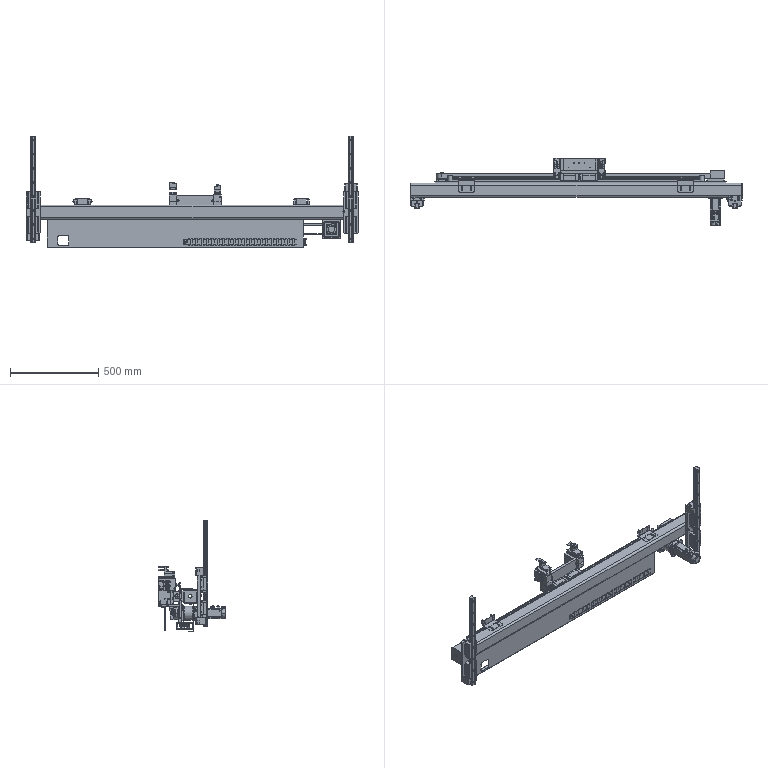Part | SolidWorks | 117 solids | 7480 faces | volume 12103229 mm3 | plane 3448 | cylinder 3339 | cone 533 | torus 120 | spline 31 | sphere 9 | commonest cylinder face diameters 1 x361 6 x301 1.1 x156 0.5 x148 6.55 x136 9 x136